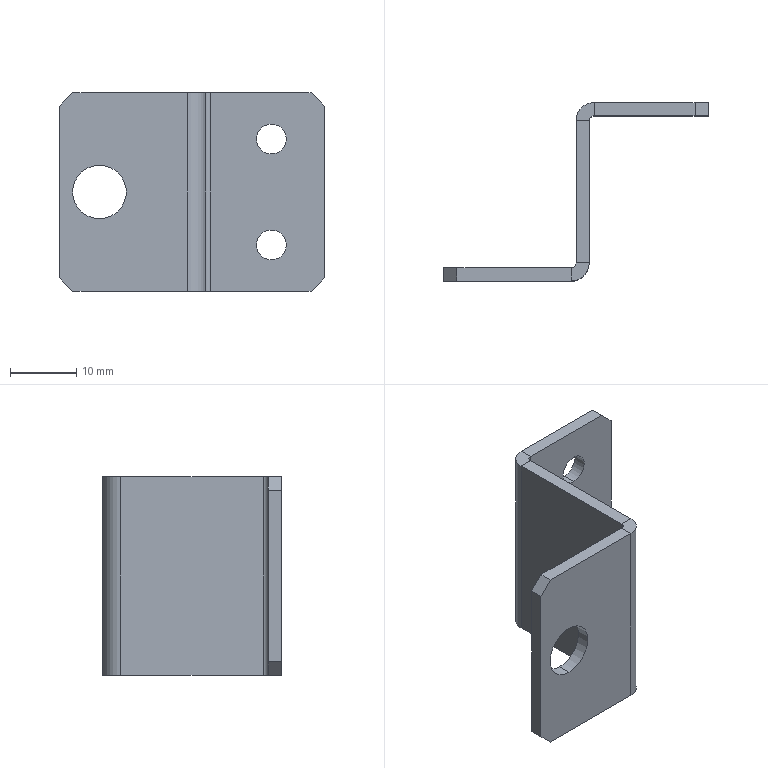Part | STEP file | 11-FG-SJ01211 | 1 solid | 32 faces | box 40 x 27 x 30 mm | volume 3628 mm3 | plane 22 | cylinder 10 | commonest cylinder face diameters 4.5 x4 1.473 x2 5.473 x2 8.1 x2
STEP:
#1=CARTESIAN_POINT('',(32.,23.,4.75));
#2=VERTEX_POINT('',#1);
#3=CARTESIAN_POINT('',(32.,23.,9.25));
#4=VERTEX_POINT('',#3);
#5=CARTESIAN_POINT('',(32.,23.,7.));
#6=DIRECTION('',(0.,1.,0.));
#7=DIRECTION('',(0.,0.,1.));
#8=AXIS2_PLACEMENT_3D('',#5,#6,#7);
#9=CIRCLE('',#8,2.25);
#10=EDGE_CURVE('',#2,#4,#9,.T.);
#11=ORIENTED_EDGE('',*,*,#10,.F.);
#12=CARTESIAN_POINT('',(32.,25.,4.75));
#13=VERTEX_POINT('',#12);
#14=CARTESIAN_POINT('',(32.,25.,4.75));
#15=DIRECTION('',(0.,1.,0.));
#16=VECTOR('',#15,1000.);
#17=LINE('',#14,#16);
#18=EDGE_CURVE('',#2,#13,#17,.T.);
#19=ORIENTED_EDGE('',*,*,#18,.T.);
#20=CARTESIAN_POINT('',(32.,25.,9.25));
#21=VERTEX_POINT('',#20);
#22=CARTESIAN_POINT('',(32.,25.,7.));
#23=DIRECTION('',(0.,1.,0.));
#24=DIRECTION('',(0.,0.,1.));
#25=AXIS2_PLACEMENT_3D('',#22,#23,#24);
#26=CIRCLE('',#25,2.25);
#27=EDGE_CURVE('',#13,#21,#26,.T.);
#28=ORIENTED_EDGE('',*,*,#27,.T.);
#29=CARTESIAN_POINT('',(32.,25.,9.25));
#30=DIRECTION('',(0.,1.,0.));
#31=VECTOR('',#30,1000.);
#32=LINE('',#29,#31);
#33=EDGE_CURVE('',#4,#21,#32,.T.);
#34=ORIENTED_EDGE('',*,*,#33,.F.);
#35=EDGE_LOOP('',(#11,#19,#28,#34));
#36=FACE_OUTER_BOUND('',#35,.T.);
#37=CARTESIAN_POINT('',(32.,25.,7.));
#38=DIRECTION('',(0.,1.,0.));
#39=DIRECTION('',(0.,0.,1.));
#40=AXIS2_PLACEMENT_3D('',#37,#38,#39);
#41=CYLINDRICAL_SURFACE('',#40,2.25);
#42=ADVANCED_FACE('',(#36),#41,.F.);
#43=CARTESIAN_POINT('',(32.,23.,20.75));
#44=VERTEX_POINT('',#43);
#45=CARTESIAN_POINT('',(32.,23.,25.25));
#46=VERTEX_POINT('',#45);
#47=CARTESIAN_POINT('',(32.,23.,23.));
#48=DIRECTION('',(0.,1.,0.));
#49=DIRECTION('',(0.,0.,1.));
#50=AXIS2_PLACEMENT_3D('',#47,#48,#49);
#51=CIRCLE('',#50,2.25);
#52=EDGE_CURVE('',#44,#46,#51,.T.);
#53=ORIENTED_EDGE('',*,*,#52,.F.);
#54=CARTESIAN_POINT('',(32.,25.,20.75));
#55=VERTEX_POINT('',#54);
#56=CARTESIAN_POINT('',(32.,25.,20.75));
#57=DIRECTION('',(0.,1.,0.));
#58=VECTOR('',#57,1000.);
#59=LINE('',#56,#58);
#60=EDGE_CURVE('',#44,#55,#59,.T.);
#61=ORIENTED_EDGE('',*,*,#60,.T.);
#62=CARTESIAN_POINT('',(32.,25.,25.25));
#63=VERTEX_POINT('',#62);
#64=CARTESIAN_POINT('',(32.,25.,23.));
#65=DIRECTION('',(0.,1.,0.));
#66=DIRECTION('',(0.,0.,1.));
#67=AXIS2_PLACEMENT_3D('',#64,#65,#66);
#68=CIRCLE('',#67,2.25);
#69=EDGE_CURVE('',#55,#63,#68,.T.);
#70=ORIENTED_EDGE('',*,*,#69,.T.);
#71=CARTESIAN_POINT('',(32.,25.,25.25));
#72=DIRECTION('',(0.,1.,0.));
#73=VECTOR('',#72,1000.);
#74=LINE('',#71,#73);
#75=EDGE_CURVE('',#46,#63,#74,.T.);
#76=ORIENTED_EDGE('',*,*,#75,.F.);
#77=EDGE_LOOP('',(#53,#61,#70,#76));
#78=FACE_OUTER_BOUND('',#77,.T.);
#79=CARTESIAN_POINT('',(32.,25.,23.));
#80=DIRECTION('',(0.,1.,0.));
#81=DIRECTION('',(0.,0.,1.));
#82=AXIS2_PLACEMENT_3D('',#79,#80,#81);
#83=CYLINDRICAL_SURFACE('',#82,2.25);
#84=ADVANCED_FACE('',(#78),#83,.F.);
#85=CARTESIAN_POINT('',(6.,0.,10.95));
#86=VERTEX_POINT('',#85);
#87=CARTESIAN_POINT('',(6.,0.,19.05));
#88=VERTEX_POINT('',#87);
#89=CARTESIAN_POINT('',(6.,0.,15.));
#90=DIRECTION('',(0.,1.,0.));
#91=DIRECTION('',(0.,0.,1.));
#92=AXIS2_PLACEMENT_3D('',#89,#90,#91);
#93=CIRCLE('',#92,4.05);
#94=EDGE_CURVE('',#86,#88,#93,.T.);
#95=ORIENTED_EDGE('',*,*,#94,.T.);
#96=CARTESIAN_POINT('',(6.,-2.,19.05));
#97=VERTEX_POINT('',#96);
#98=CARTESIAN_POINT('',(6.,8.,19.05));
#99=DIRECTION('',(0.,-1.,0.));
#100=VECTOR('',#99,1000.);
#101=LINE('',#98,#100);
#102=EDGE_CURVE('',#88,#97,#101,.T.);
#103=ORIENTED_EDGE('',*,*,#102,.T.);
#104=CARTESIAN_POINT('',(6.,-2.,10.95));
#105=VERTEX_POINT('',#104);
#106=CARTESIAN_POINT('',(6.,-2.,15.));
#107=DIRECTION('',(0.,-1.,0.));
#108=DIRECTION('',(0.,0.,-1.));
#109=AXIS2_PLACEMENT_3D('',#106,#107,#108);
#110=CIRCLE('',#109,4.05);
#111=EDGE_CURVE('',#97,#105,#110,.T.);
#112=ORIENTED_EDGE('',*,*,#111,.T.);
#113=CARTESIAN_POINT('',(6.,8.,10.95));
#114=DIRECTION('',(0.,-1.,0.));
#115=VECTOR('',#114,1000.);
#116=LINE('',#113,#115);
#117=EDGE_CURVE('',#86,#105,#116,.T.);
#118=ORIENTED_EDGE('',*,*,#117,.F.);
#119=EDGE_LOOP('',(#95,#103,#112,#118));
#120=FACE_OUTER_BOUND('',#119,.T.);
#121=CARTESIAN_POINT('',(6.,8.,15.));
#122=DIRECTION('',(0.,-1.,0.));
#123=DIRECTION('',(0.,0.,-1.));
#124=AXIS2_PLACEMENT_3D('',#121,#122,#123);
#125=CYLINDRICAL_SURFACE('',#124,4.05);
#126=ADVANCED_FACE('',(#120),#125,.F.);
#127=CARTESIAN_POINT('',(20.,0.7366,30.));
#128=VERTEX_POINT('',#127);
#129=CARTESIAN_POINT('',(22.,0.7366,30.));
#130=VERTEX_POINT('',#129);
#131=CARTESIAN_POINT('',(20.,0.7366,30.));
#132=DIRECTION('',(1.,0.,0.));
#133=VECTOR('',#132,1000.);
#134=LINE('',#131,#133);
#135=EDGE_CURVE('',#128,#130,#134,.T.);
#136=ORIENTED_EDGE('',*,*,#135,.F.);
#137=CARTESIAN_POINT('',(19.263,0.,30.));
#138=VERTEX_POINT('',#137);
#139=CARTESIAN_POINT('',(19.263,0.7366,30.));
#140=DIRECTION('',(0.,0.,1.));
#141=DIRECTION('',(-1.,0.,0.));
#142=AXIS2_PLACEMENT_3D('',#139,#140,#141);
#143=CIRCLE('',#142,0.7366);
#144=EDGE_CURVE('',#138,#128,#143,.T.);
#145=ORIENTED_EDGE('',*,*,#144,.F.);
#146=CARTESIAN_POINT('',(19.263,-2.,30.));
#147=VERTEX_POINT('',#146);
#148=CARTESIAN_POINT('',(19.263,-2.,30.));
#149=DIRECTION('',(0.,1.,0.));
#150=VECTOR('',#149,1000.);
#151=LINE('',#148,#150);
#152=EDGE_CURVE('',#147,#138,#151,.T.);
#153=ORIENTED_EDGE('',*,*,#152,.F.);
#154=CARTESIAN_POINT('',(19.263,0.7366,30.));
#155=DIRECTION('',(0.,0.,1.));
#156=DIRECTION('',(1.,0.,0.));
#157=AXIS2_PLACEMENT_3D('',#154,#155,#156);
#158=CIRCLE('',#157,2.737);
#159=EDGE_CURVE('',#147,#130,#158,.T.);
#160=ORIENTED_EDGE('',*,*,#159,.T.);
#161=EDGE_LOOP('',(#136,#145,#153,#160));
#162=FACE_OUTER_BOUND('',#161,.T.);
#163=CARTESIAN_POINT('',(20.,0.7366,30.));
#164=DIRECTION('',(0.,0.,1.));
#165=DIRECTION('',(1.,0.,0.));
#166=AXIS2_PLACEMENT_3D('',#163,#164,#165);
#167=PLANE('',#166);
#168=ADVANCED_FACE('',(#162),#167,.T.);
#169=CARTESIAN_POINT('',(20.,22.263,30.));
#170=VERTEX_POINT('',#169);
#171=CARTESIAN_POINT('',(20.,0.,30.));
#172=DIRECTION('',(0.,1.,0.));
#173=VECTOR('',#172,1000.);
#174=LINE('',#171,#173);
#175=EDGE_CURVE('',#128,#170,#174,.T.);
#176=ORIENTED_EDGE('',*,*,#175,.F.);
#177=ORIENTED_EDGE('',*,*,#135,.T.);
#178=CARTESIAN_POINT('',(22.,22.263,30.));
#179=VERTEX_POINT('',#178);
#180=CARTESIAN_POINT('',(22.,0.,30.));
#181=DIRECTION('',(0.,1.,0.));
#182=VECTOR('',#181,1000.);
#183=LINE('',#180,#182);
#184=EDGE_CURVE('',#130,#179,#183,.T.);
#185=ORIENTED_EDGE('',*,*,#184,.T.);
#186=CARTESIAN_POINT('',(22.,22.263,30.));
#187=DIRECTION('',(-1.,0.,0.));
#188=VECTOR('',#187,1000.);
#189=LINE('',#186,#188);
#190=EDGE_CURVE('',#179,#170,#189,.T.);
#191=ORIENTED_EDGE('',*,*,#190,.T.);
#192=EDGE_LOOP('',(#176,#177,#185,#191));
#193=FACE_OUTER_BOUND('',#192,.T.);
#194=CARTESIAN_POINT('',(19.263,-2.,30.));
#195=DIRECTION('',(0.,0.,1.));
#196=DIRECTION('',(1.,0.,0.));
#197=AXIS2_PLACEMENT_3D('',#194,#195,#196);
#198=PLANE('',#197);
#199=ADVANCED_FACE('',(#193),#198,.T.);
#200=CARTESIAN_POINT('',(19.263,0.,0.));
#201=VERTEX_POINT('',#200);
#202=CARTESIAN_POINT('',(19.263,-2.,0.));
#203=VERTEX_POINT('',#202);
#204=CARTESIAN_POINT('',(19.263,0.,0.));
#205=DIRECTION('',(0.,-1.,0.));
#206=VECTOR('',#205,1000.);
#207=LINE('',#204,#206);
#208=EDGE_CURVE('',#201,#203,#207,.T.);
#209=ORIENTED_EDGE('',*,*,#208,.F.);
#210=CARTESIAN_POINT('',(20.,0.7366,0.));
#211=VERTEX_POINT('',#210);
#212=CARTESIAN_POINT('',(19.263,0.7366,0.));
#213=DIRECTION('',(0.,0.,1.));
#214=DIRECTION('',(-1.,0.,0.));
#215=AXIS2_PLACEMENT_3D('',#212,#213,#214);
#216=CIRCLE('',#215,0.7366);
#217=EDGE_CURVE('',#201,#211,#216,.T.);
#218=ORIENTED_EDGE('',*,*,#217,.T.);
#219=CARTESIAN_POINT('',(22.,0.7366,0.));
#220=VERTEX_POINT('',#219);
#221=CARTESIAN_POINT('',(22.,0.7366,0.));
#222=DIRECTION('',(-1.,0.,0.));
#223=VECTOR('',#222,1000.);
#224=LINE('',#221,#223);
#225=EDGE_CURVE('',#220,#211,#224,.T.);
#226=ORIENTED_EDGE('',*,*,#225,.F.);
#227=CARTESIAN_POINT('',(19.263,0.7366,0.));
#228=DIRECTION('',(0.,0.,1.));
#229=DIRECTION('',(1.,0.,0.));
#230=AXIS2_PLACEMENT_3D('',#227,#228,#229);
#231=CIRCLE('',#230,2.737);
#232=EDGE_CURVE('',#203,#220,#231,.T.);
#233=ORIENTED_EDGE('',*,*,#232,.F.);
#234=EDGE_LOOP('',(#209,#218,#226,#233));
#235=FACE_OUTER_BOUND('',#234,.T.);
#236=CARTESIAN_POINT('',(19.263,0.,0.));
#237=DIRECTION('',(0.,0.,-1.));
#238=DIRECTION('',(-1.,0.,0.));
#239=AXIS2_PLACEMENT_3D('',#236,#237,#238);
#240=PLANE('',#239);
#241=ADVANCED_FACE('',(#235),#240,.T.);
#242=CARTESIAN_POINT('',(2.,-2.,0.));
#243=VERTEX_POINT('',#242);
#244=CARTESIAN_POINT('',(0.,-2.,0.));
#245=DIRECTION('',(1.,0.,0.));
#246=VECTOR('',#245,1000.);
#247=LINE('',#244,#246);
#248=EDGE_CURVE('',#243,#203,#247,.T.);
#249=ORIENTED_EDGE('',*,*,#248,.F.);
#250=CARTESIAN_POINT('',(2.,0.,0.));
#251=VERTEX_POINT('',#250);
#252=CARTESIAN_POINT('',(2.,0.7366,0.));
#253=DIRECTION('',(0.,1.,0.));
#254=VECTOR('',#253,1000.);
#255=LINE('',#252,#254);
#256=EDGE_CURVE('',#243,#251,#255,.T.);
#257=ORIENTED_EDGE('',*,*,#256,.T.);
#258=CARTESIAN_POINT('',(0.,0.,0.));
#259=DIRECTION('',(1.,0.,0.));
#260=VECTOR('',#259,1000.);
#261=LINE('',#258,#260);
#262=EDGE_CURVE('',#251,#201,#261,.T.);
#263=ORIENTED_EDGE('',*,*,#262,.T.);
#264=ORIENTED_EDGE('',*,*,#208,.T.);
#265=EDGE_LOOP('',(#249,#257,#263,#264));
#266=FACE_OUTER_BOUND('',#265,.T.);
#267=CARTESIAN_POINT('',(22.,0.7366,0.));
#268=DIRECTION('',(0.,0.,-1.));
#269=DIRECTION('',(-1.,0.,0.));
#270=AXIS2_PLACEMENT_3D('',#267,#268,#269);
#271=PLANE('',#270);
#272=ADVANCED_FACE('',(#266),#271,.T.);
#273=CARTESIAN_POINT('',(22.737,25.,30.));
#274=VERTEX_POINT('',#273);
#275=CARTESIAN_POINT('',(22.737,23.,30.));
#276=VERTEX_POINT('',#275);
#277=CARTESIAN_POINT('',(22.737,25.,30.));
#278=DIRECTION('',(0.,-1.,0.));
#279=VECTOR('',#278,1000.);
#280=LINE('',#277,#279);
#281=EDGE_CURVE('',#274,#276,#280,.T.);
#282=ORIENTED_EDGE('',*,*,#281,.F.);
#283=CARTESIAN_POINT('',(22.737,22.263,30.));
#284=DIRECTION('',(0.,0.,-1.));
#285=DIRECTION('',(1.,0.,0.));
#286=AXIS2_PLACEMENT_3D('',#283,#284,#285);
#287=CIRCLE('',#286,2.737);
#288=EDGE_CURVE('',#170,#274,#287,.T.);
#289=ORIENTED_EDGE('',*,*,#288,.F.);
#290=ORIENTED_EDGE('',*,*,#190,.F.);
#291=CARTESIAN_POINT('',(22.737,22.263,30.));
#292=DIRECTION('',(0.,0.,-1.));
#293=DIRECTION('',(1.,0.,0.));
#294=AXIS2_PLACEMENT_3D('',#291,#292,#293);
#295=CIRCLE('',#294,0.7366);
#296=EDGE_CURVE('',#179,#276,#295,.T.);
#297=ORIENTED_EDGE('',*,*,#296,.T.);
#298=EDGE_LOOP('',(#282,#289,#290,#297));
#299=FACE_OUTER_BOUND('',#298,.T.);
#300=CARTESIAN_POINT('',(22.737,25.,30.));
#301=DIRECTION('',(0.,0.,1.));
#302=DIRECTION('',(1.,0.,0.));
#303=AXIS2_PLACEMENT_3D('',#300,#301,#302);
#304=PLANE('',#303);
#305=ADVANCED_FACE('',(#299),#304,.T.);
#306=CARTESIAN_POINT('',(38.,23.,30.));
#307=VERTEX_POINT('',#306);
#308=CARTESIAN_POINT('',(20.,23.,30.));
#309=DIRECTION('',(1.,0.,0.));
#310=VECTOR('',#309,1000.);
#311=LINE('',#308,#310);
#312=EDGE_CURVE('',#276,#307,#311,.T.);
#313=ORIENTED_EDGE('',*,*,#312,.T.);
#314=CARTESIAN_POINT('',(38.,25.,30.));
#315=VERTEX_POINT('',#314);
#316=CARTESIAN_POINT('',(38.,22.263,30.));
#317=DIRECTION('',(0.,1.,0.));
#318=VECTOR('',#317,1000.);
#319=LINE('',#316,#318);
#320=EDGE_CURVE('',#307,#315,#319,.T.);
#321=ORIENTED_EDGE('',*,*,#320,.T.);
#322=CARTESIAN_POINT('',(20.,25.,30.));
#323=DIRECTION('',(1.,0.,0.));
#324=VECTOR('',#323,1000.);
#325=LINE('',#322,#324);
#326=EDGE_CURVE('',#274,#315,#325,.T.);
#327=ORIENTED_EDGE('',*,*,#326,.F.);
#328=ORIENTED_EDGE('',*,*,#281,.T.);
#329=EDGE_LOOP('',(#313,#321,#327,#328));
#330=FACE_OUTER_BOUND('',#329,.T.);
#331=CARTESIAN_POINT('',(22.,22.263,30.));
#332=DIRECTION('',(0.,0.,1.));
#333=DIRECTION('',(1.,0.,0.));
#334=AXIS2_PLACEMENT_3D('',#331,#332,#333);
#335=PLANE('',#334);
#336=ADVANCED_FACE('',(#330),#335,.T.);
#337=CARTESIAN_POINT('',(20.,22.263,0.));
#338=VERTEX_POINT('',#337);
#339=CARTESIAN_POINT('',(22.,22.263,0.));
#340=VERTEX_POINT('',#339);
#341=CARTESIAN_POINT('',(20.,22.263,0.));
#342=DIRECTION('',(1.,0.,0.));
#343=VECTOR('',#342,1000.);
#344=LINE('',#341,#343);
#345=EDGE_CURVE('',#338,#340,#344,.T.);
#346=ORIENTED_EDGE('',*,*,#345,.F.);
#347=CARTESIAN_POINT('',(22.737,25.,0.));
#348=VERTEX_POINT('',#347);
#349=CARTESIAN_POINT('',(22.737,22.263,0.));
#350=DIRECTION('',(0.,0.,-1.));
#351=DIRECTION('',(1.,0.,0.));
#352=AXIS2_PLACEMENT_3D('',#349,#350,#351);
#353=CIRCLE('',#352,2.737);
#354=EDGE_CURVE('',#338,#348,#353,.T.);
#355=ORIENTED_EDGE('',*,*,#354,.T.);
#356=CARTESIAN_POINT('',(22.737,23.,0.));
#357=VERTEX_POINT('',#356);
#358=CARTESIAN_POINT('',(22.737,23.,0.));
#359=DIRECTION('',(0.,1.,0.));
#360=VECTOR('',#359,1000.);
#361=LINE('',#358,#360);
#362=EDGE_CURVE('',#357,#348,#361,.T.);
#363=ORIENTED_EDGE('',*,*,#362,.F.);
#364=CARTESIAN_POINT('',(22.737,22.263,0.));
#365=DIRECTION('',(0.,0.,-1.));
#366=DIRECTION('',(1.,0.,0.));
#367=AXIS2_PLACEMENT_3D('',#364,#365,#366);
#368=CIRCLE('',#367,0.7366);
#369=EDGE_CURVE('',#340,#357,#368,.T.);
#370=ORIENTED_EDGE('',*,*,#369,.F.);
#371=EDGE_LOOP('',(#346,#355,#363,#370));
#372=FACE_OUTER_BOUND('',#371,.T.);
#373=CARTESIAN_POINT('',(20.,22.263,0.));
#374=DIRECTION('',(0.,0.,-1.));
#375=DIRECTION('',(-1.,0.,0.));
#376=AXIS2_PLACEMENT_3D('',#373,#374,#375);
#377=PLANE('',#376);
#378=ADVANCED_FACE('',(#372),#377,.T.);
#379=CARTESIAN_POINT('',(20.,0.,0.));
#380=DIRECTION('',(0.,1.,0.));
#381=VECTOR('',#380,1000.);
#382=LINE('',#379,#381);
#383=EDGE_CURVE('',#211,#338,#382,.T.);
#384=ORIENTED_EDGE('',*,*,#383,.T.);
#385=ORIENTED_EDGE('',*,*,#345,.T.);
#386=CARTESIAN_POINT('',(22.,0.,0.));
#387=DIRECTION('',(0.,1.,0.));
#388=VECTOR('',#387,1000.);
#389=LINE('',#386,#388);
#390=EDGE_CURVE('',#220,#340,#389,.T.);
#391=ORIENTED_EDGE('',*,*,#390,.F.);
#392=ORIENTED_EDGE('',*,*,#225,.T.);
#393=EDGE_LOOP('',(#384,#385,#391,#392));
#394=FACE_OUTER_BOUND('',#393,.T.);
#395=CARTESIAN_POINT('',(22.737,23.,0.));
#396=DIRECTION('',(0.,0.,-1.));
#397=DIRECTION('',(-1.,0.,0.));
#398=AXIS2_PLACEMENT_3D('',#395,#396,#397);
#399=PLANE('',#398);
#400=ADVANCED_FACE('',(#394),#399,.T.);
#401=CARTESIAN_POINT('',(32.,23.,7.));
#402=DIRECTION('',(0.,1.,0.));
#403=DIRECTION('',(0.,0.,1.));
#404=AXIS2_PLACEMENT_3D('',#401,#402,#403);
#405=CIRCLE('',#404,2.25);
#406=EDGE_CURVE('',#4,#2,#405,.T.);
#407=ORIENTED_EDGE('',*,*,#406,.T.);
#408=ORIENTED_EDGE('',*,*,#10,.T.);
#409=EDGE_LOOP('',(#407,#408));
#410=FACE_BOUND('',#409,.T.);
#411=CARTESIAN_POINT('',(32.,23.,23.));
#412=DIRECTION('',(0.,1.,0.));
#413=DIRECTION('',(0.,0.,1.));
#414=AXIS2_PLACEMENT_3D('',#411,#412,#413);
#415=CIRCLE('',#414,2.25);
#416=EDGE_CURVE('',#46,#44,#415,.T.);
#417=ORIENTED_EDGE('',*,*,#416,.T.);
#418=ORIENTED_EDGE('',*,*,#52,.T.);
#419=EDGE_LOOP('',(#417,#418));
#420=FACE_BOUND('',#419,.T.);
#421=CARTESIAN_POINT('',(38.,23.,0.));
#422=VERTEX_POINT('',#421);
#423=CARTESIAN_POINT('',(20.,23.,0.));
#424=DIRECTION('',(1.,0.,0.));
#425=VECTOR('',#424,1000.);
#426=LINE('',#423,#425);
#427=EDGE_CURVE('',#357,#422,#426,.T.);
#428=ORIENTED_EDGE('',*,*,#427,.T.);
#429=CARTESIAN_POINT('',(40.,23.,2.));
#430=VERTEX_POINT('',#429);
#431=CARTESIAN_POINT('',(38.,23.,0.));
#432=DIRECTION('',(0.7071,0.,0.7071));
#433=VECTOR('',#432,1000.);
#434=LINE('',#431,#433);
#435=EDGE_CURVE('',#422,#430,#434,.T.);
#436=ORIENTED_EDGE('',*,*,#435,.T.);
#437=CARTESIAN_POINT('',(40.,23.,28.));
#438=VERTEX_POINT('',#437);
#439=CARTESIAN_POINT('',(40.,23.,30.));
#440=DIRECTION('',(0.,0.,-1.));
#441=VECTOR('',#440,1000.);
#442=LINE('',#439,#441);
#443=EDGE_CURVE('',#438,#430,#442,.T.);
#444=ORIENTED_EDGE('',*,*,#443,.F.);
#445=CARTESIAN_POINT('',(40.,23.,28.));
#446=DIRECTION('',(-0.7071,0.,0.7071));
#447=VECTOR('',#446,1000.);
#448=LINE('',#445,#447);
#449=EDGE_CURVE('',#438,#307,#448,.T.);
#450=ORIENTED_EDGE('',*,*,#449,.T.);
#451=ORIENTED_EDGE('',*,*,#312,.F.);
#452=CARTESIAN_POINT('',(22.737,23.,30.));
#453=DIRECTION('',(0.,0.,-1.));
#454=VECTOR('',#453,1000.);
#455=LINE('',#452,#454);
#456=EDGE_CURVE('',#276,#357,#455,.T.);
#457=ORIENTED_EDGE('',*,*,#456,.T.);
#458=EDGE_LOOP('',(#428,#436,#444,#450,#451,#457));
#459=FACE_OUTER_BOUND('',#458,.T.);
#460=CARTESIAN_POINT('',(20.,23.,30.));
#461=DIRECTION('',(0.,1.,0.));
#462=DIRECTION('',(0.,0.,1.));
#463=AXIS2_PLACEMENT_3D('',#460,#461,#462);
#464=PLANE('',#463);
#465=ADVANCED_FACE('',(#410,#420,#459),#464,.F.);
#466=ORIENTED_EDGE('',*,*,#443,.T.);
#467=CARTESIAN_POINT('',(40.,25.,2.));
#468=VERTEX_POINT('',#467);
#469=CARTESIAN_POINT('',(40.,25.,2.));
#470=DIRECTION('',(0.,1.,0.));
#471=VECTOR('',#470,1000.);
#472=LINE('',#469,#471);
#473=EDGE_CURVE('',#430,#468,#472,.T.);
#474=ORIENTED_EDGE('',*,*,#473,.T.);
#475=CARTESIAN_POINT('',(40.,25.,28.));
#476=VERTEX_POINT('',#475);
#477=CARTESIAN_POINT('',(40.,25.,30.));
#478=DIRECTION('',(0.,0.,-1.));
#479=VECTOR('',#478,1000.);
#480=LINE('',#477,#479);
#481=EDGE_CURVE('',#476,#468,#480,.T.);
#482=ORIENTED_EDGE('',*,*,#481,.F.);
#483=CARTESIAN_POINT('',(40.,25.,28.));
#484=DIRECTION('',(0.,-1.,0.));
#485=VECTOR('',#484,1000.);
#486=LINE('',#483,#485);
#487=EDGE_CURVE('',#476,#438,#486,.T.);
#488=ORIENTED_EDGE('',*,*,#487,.T.);
#489=EDGE_LOOP('',(#466,#474,#482,#488));
#490=FACE_OUTER_BOUND('',#489,.T.);
#491=CARTESIAN_POINT('',(40.,25.,30.));
#492=DIRECTION('',(1.,0.,0.));
#493=DIRECTION('',(0.,0.,-1.));
#494=AXIS2_PLACEMENT_3D('',#491,#492,#493);
#495=PLANE('',#494);
#496=ADVANCED_FACE('',(#490),#495,.T.);
#497=CARTESIAN_POINT('',(32.,25.,7.));
#498=DIRECTION('',(0.,1.,0.));
#499=DIRECTION('',(0.,0.,1.));
#500=AXIS2_PLACEMENT_3D('',#497,#498,#499);
#501=CIRCLE('',#500,2.25);
#502=EDGE_CURVE('',#21,#13,#501,.T.);
#503=ORIENTED_EDGE('',*,*,#502,.F.);
#504=ORIENTED_EDGE('',*,*,#27,.F.);
#505=EDGE_LOOP('',(#503,#504));
#506=FACE_BOUND('',#505,.T.);
#507=CARTESIAN_POINT('',(32.,25.,23.));
#508=DIRECTION('',(0.,1.,0.));
#509=DIRECTION('',(0.,0.,1.));
#510=AXIS2_PLACEMENT_3D('',#507,#508,#509);
#511=CIRCLE('',#510,2.25);
#512=EDGE_CURVE('',#63,#55,#511,.T.);
#513=ORIENTED_EDGE('',*,*,#512,.F.);
#514=ORIENTED_EDGE('',*,*,#69,.F.);
#515=EDGE_LOOP('',(#513,#514));
#516=FACE_BOUND('',#515,.T.);
#517=ORIENTED_EDGE('',*,*,#481,.T.);
#518=CARTESIAN_POINT('',(38.,25.,0.));
#519=VERTEX_POINT('',#518);
#520=CARTESIAN_POINT('',(44.,25.,6.));
#521=DIRECTION('',(-0.7071,0.,-0.7071));
#522=VECTOR('',#521,1000.);
#523=LINE('',#520,#522);
#524=EDGE_CURVE('',#468,#519,#523,.T.);
#525=ORIENTED_EDGE('',*,*,#524,.T.);
#526=CARTESIAN_POINT('',(20.,25.,0.));
#527=DIRECTION('',(1.,0.,0.));
#528=VECTOR('',#527,1000.);
#529=LINE('',#526,#528);
#530=EDGE_CURVE('',#348,#519,#529,.T.);
#531=ORIENTED_EDGE('',*,*,#530,.F.);
#532=CARTESIAN_POINT('',(22.737,25.,30.));
#533=DIRECTION('',(0.,0.,-1.));
#534=VECTOR('',#533,1000.);
#535=LINE('',#532,#534);
#536=EDGE_CURVE('',#274,#348,#535,.T.);
#537=ORIENTED_EDGE('',*,*,#536,.F.);
#538=ORIENTED_EDGE('',*,*,#326,.T.);
#539=CARTESIAN_POINT('',(29.,25.,39.));
#540=DIRECTION('',(0.7071,0.,-0.7071));
#541=VECTOR('',#540,1000.);
#542=LINE('',#539,#541);
#543=EDGE_CURVE('',#315,#476,#542,.T.);
#544=ORIENTED_EDGE('',*,*,#543,.T.);
#545=EDGE_LOOP('',(#517,#525,#531,#537,#538,#544));
#546=FACE_OUTER_BOUND('',#545,.T.);
#547=CARTESIAN_POINT('',(20.,25.,30.));
#548=DIRECTION('',(0.,1.,0.));
#549=DIRECTION('',(0.,0.,1.));
#550=AXIS2_PLACEMENT_3D('',#547,#548,#549);
#551=PLANE('',#550);
#552=ADVANCED_FACE('',(#506,#516,#546),#551,.T.);
#553=ORIENTED_EDGE('',*,*,#354,.F.);
#554=CARTESIAN_POINT('',(20.,22.263,30.));
#555=DIRECTION('',(0.,0.,-1.));
#556=VECTOR('',#555,1000.);
#557=LINE('',#554,#556);
#558=EDGE_CURVE('',#170,#338,#557,.T.);
#559=ORIENTED_EDGE('',*,*,#558,.F.);
#560=ORIENTED_EDGE('',*,*,#288,.T.);
#561=ORIENTED_EDGE('',*,*,#536,.T.);
#562=EDGE_LOOP('',(#553,#559,#560,#561));
#563=FACE_OUTER_BOUND('',#562,.T.);
#564=CARTESIAN_POINT('',(22.737,22.263,30.));
#565=DIRECTION('',(0.,0.,-1.));
#566=DIRECTION('',(-1.,0.,0.));
#567=AXIS2_PLACEMENT_3D('',#564,#565,#566);
#568=CYLINDRICAL_SURFACE('',#567,2.737);
#569=ADVANCED_FACE('',(#563),#568,.T.);
#570=ORIENTED_EDGE('',*,*,#383,.F.);
#571=CARTESIAN_POINT('',(20.,0.7366,30.));
#572=DIRECTION('',(0.,0.,-1.));
#573=VECTOR('',#572,1000.);
#574=LINE('',#571,#573);
#575=EDGE_CURVE('',#128,#211,#574,.T.);
#576=ORIENTED_EDGE('',*,*,#575,.F.);
#577=ORIENTED_EDGE('',*,*,#175,.T.);
#578=ORIENTED_EDGE('',*,*,#558,.T.);
#579=EDGE_LOOP('',(#570,#576,#577,#578));
#580=FACE_OUTER_BOUND('',#579,.T.);
#581=CARTESIAN_POINT('',(20.,0.,30.));
#582=DIRECTION('',(-1.,0.,0.));
#583=DIRECTION('',(0.,0.,1.));
#584=AXIS2_PLACEMENT_3D('',#581,#582,#583);
#585=PLANE('',#584);
#586=ADVANCED_FACE('',(#580),#585,.T.);
#587=ORIENTED_EDGE('',*,*,#217,.F.);
#588=CARTESIAN_POINT('',(19.263,0.,30.));
#589=DIRECTION('',(0.,0.,-1.));
#590=VECTOR('',#589,1000.);
#591=LINE('',#588,#590);
#592=EDGE_CURVE('',#138,#201,#591,.T.);
#593=ORIENTED_EDGE('',*,*,#592,.F.);
#594=ORIENTED_EDGE('',*,*,#144,.T.);
#595=ORIENTED_EDGE('',*,*,#575,.T.);
#596=EDGE_LOOP('',(#587,#593,#594,#595));
#597=FACE_OUTER_BOUND('',#596,.T.);
#598=CARTESIAN_POINT('',(19.263,0.7366,30.));
#599=DIRECTION('',(0.,0.,-1.));
#600=DIRECTION('',(-1.,0.,0.));
#601=AXIS2_PLACEMENT_3D('',#598,#599,#600);
#602=CYLINDRICAL_SURFACE('',#601,0.7366);
#603=ADVANCED_FACE('',(#597),#602,.F.);
#604=ORIENTED_EDGE('',*,*,#94,.F.);
#605=CARTESIAN_POINT('',(6.,0.,15.));
#606=DIRECTION('',(0.,1.,0.));
#607=DIRECTION('',(0.,0.,1.));
#608=AXIS2_PLACEMENT_3D('',#605,#606,#607);
#609=CIRCLE('',#608,4.05);
#610=EDGE_CURVE('',#88,#86,#609,.T.);
#611=ORIENTED_EDGE('',*,*,#610,.F.);
#612=EDGE_LOOP('',(#604,#611));
#613=FACE_BOUND('',#612,.T.);
#614=ORIENTED_EDGE('',*,*,#262,.F.);
#615=CARTESIAN_POINT('',(0.,0.,2.));
#616=VERTEX_POINT('',#615);
#617=CARTESIAN_POINT('',(-14.,0.,16.));
#618=DIRECTION('',(-0.7071,0.,0.7071));
#619=VECTOR('',#618,1000.);
#620=LINE('',#617,#619);
#621=EDGE_CURVE('',#251,#616,#620,.T.);
#622=ORIENTED_EDGE('',*,*,#621,.T.);
#623=CARTESIAN_POINT('',(0.,0.,28.));
#624=VERTEX_POINT('',#623);
#625=CARTESIAN_POINT('',(0.,0.,30.));
#626=DIRECTION('',(0.,0.,-1.));
#627=VECTOR('',#626,1000.);
#628=LINE('',#625,#627);
#629=EDGE_CURVE('',#624,#616,#628,.T.);
#630=ORIENTED_EDGE('',*,*,#629,.F.);
#631=CARTESIAN_POINT('',(2.,0.,30.));
#632=VERTEX_POINT('',#631);
#633=CARTESIAN_POINT('',(1.,0.,29.));
#634=DIRECTION('',(0.7071,0.,0.7071));
#635=VECTOR('',#634,1000.);
#636=LINE('',#633,#635);
#637=EDGE_CURVE('',#624,#632,#636,.T.);
#638=ORIENTED_EDGE('',*,*,#637,.T.);
#639=CARTESIAN_POINT('',(0.,0.,30.));
#640=DIRECTION('',(1.,0.,0.));
#641=VECTOR('',#640,1000.);
#642=LINE('',#639,#641);
#643=EDGE_CURVE('',#632,#138,#642,.T.);
#644=ORIENTED_EDGE('',*,*,#643,.T.);
#645=ORIENTED_EDGE('',*,*,#592,.T.);
#646=EDGE_LOOP('',(#614,#622,#630,#638,#644,#645));
#647=FACE_OUTER_BOUND('',#646,.T.);
#648=CARTESIAN_POINT('',(0.,0.,30.));
#649=DIRECTION('',(0.,1.,0.));
#650=DIRECTION('',(0.,0.,1.));
#651=AXIS2_PLACEMENT_3D('',#648,#649,#650);
#652=PLANE('',#651);
#653=ADVANCED_FACE('',(#613,#647),#652,.T.);
#654=ORIENTED_EDGE('',*,*,#629,.T.);
#655=CARTESIAN_POINT('',(0.,-2.,2.));
#656=VERTEX_POINT('',#655);
#657=CARTESIAN_POINT('',(0.,-2.,2.));
#658=DIRECTION('',(0.,-1.,0.));
#659=VECTOR('',#658,1000.);
#660=LINE('',#657,#659);
#661=EDGE_CURVE('',#616,#656,#660,.T.);
#662=ORIENTED_EDGE('',*,*,#661,.T.);
#663=CARTESIAN_POINT('',(0.,-2.,28.));
#664=VERTEX_POINT('',#663);
#665=CARTESIAN_POINT('',(0.,-2.,30.));
#666=DIRECTION('',(0.,0.,-1.));
#667=VECTOR('',#666,1000.);
#668=LINE('',#665,#667);
#669=EDGE_CURVE('',#664,#656,#668,.T.);
#670=ORIENTED_EDGE('',*,*,#669,.F.);
#671=CARTESIAN_POINT('',(0.,-2.,28.));
#672=DIRECTION('',(0.,1.,0.));
#673=VECTOR('',#672,1000.);
#674=LINE('',#671,#673);
#675=EDGE_CURVE('',#664,#624,#674,.T.);
#676=ORIENTED_EDGE('',*,*,#675,.T.);
#677=EDGE_LOOP('',(#654,#662,#670,#676));
#678=FACE_OUTER_BOUND('',#677,.T.);
#679=CARTESIAN_POINT('',(0.,-2.,30.));
#680=DIRECTION('',(-1.,0.,0.));
#681=DIRECTION('',(0.,0.,1.));
#682=AXIS2_PLACEMENT_3D('',#679,#680,#681);
#683=PLANE('',#682);
#684=ADVANCED_FACE('',(#678),#683,.T.);
#685=CARTESIAN_POINT('',(6.,-2.,15.));
#686=DIRECTION('',(0.,-1.,0.));
#687=DIRECTION('',(0.,0.,-1.));
#688=AXIS2_PLACEMENT_3D('',#685,#686,#687);
#689=CIRCLE('',#688,4.05);
#690=EDGE_CURVE('',#105,#97,#689,.T.);
#691=ORIENTED_EDGE('',*,*,#690,.F.);
#692=ORIENTED_EDGE('',*,*,#111,.F.);
#693=EDGE_LOOP('',(#691,#692));
#694=FACE_BOUND('',#693,.T.);
#695=ORIENTED_EDGE('',*,*,#669,.T.);
#696=CARTESIAN_POINT('',(2.,-2.,0.));
#697=DIRECTION('',(0.7071,0.,-0.7071));
#698=VECTOR('',#697,1000.);
#699=LINE('',#696,#698);
#700=EDGE_CURVE('',#656,#243,#699,.T.);
#701=ORIENTED_EDGE('',*,*,#700,.T.);
#702=ORIENTED_EDGE('',*,*,#248,.T.);
#703=CARTESIAN_POINT('',(19.263,-2.,30.));
#704=DIRECTION('',(0.,0.,-1.));
#705=VECTOR('',#704,1000.);
#706=LINE('',#703,#705);
#707=EDGE_CURVE('',#147,#203,#706,.T.);
#708=ORIENTED_EDGE('',*,*,#707,.F.);
#709=CARTESIAN_POINT('',(2.,-2.,30.));
#710=VERTEX_POINT('',#709);
#711=CARTESIAN_POINT('',(0.,-2.,30.));
#712=DIRECTION('',(1.,0.,0.));
#713=VECTOR('',#712,1000.);
#714=LINE('',#711,#713);
#715=EDGE_CURVE('',#710,#147,#714,.T.);
#716=ORIENTED_EDGE('',*,*,#715,.F.);
#717=CARTESIAN_POINT('',(0.,-2.,28.));
#718=DIRECTION('',(-0.7071,0.,-0.7071));
#719=VECTOR('',#718,1000.);
#720=LINE('',#717,#719);
#721=EDGE_CURVE('',#710,#664,#720,.T.);
#722=ORIENTED_EDGE('',*,*,#721,.T.);
#723=EDGE_LOOP('',(#695,#701,#702,#708,#716,#722));
#724=FACE_OUTER_BOUND('',#723,.T.);
#725=CARTESIAN_POINT('',(0.,-2.,30.));
#726=DIRECTION('',(0.,1.,0.));
#727=DIRECTION('',(0.,0.,1.));
#728=AXIS2_PLACEMENT_3D('',#725,#726,#727);
#729=PLANE('',#728);
#730=ADVANCED_FACE('',(#694,#724),#729,.F.);
#731=ORIENTED_EDGE('',*,*,#232,.T.);
#732=CARTESIAN_POINT('',(22.,0.7366,30.));
#733=DIRECTION('',(0.,0.,-1.));
#734=VECTOR('',#733,1000.);
#735=LINE('',#732,#734);
#736=EDGE_CURVE('',#130,#220,#735,.T.);
#737=ORIENTED_EDGE('',*,*,#736,.F.);
#738=ORIENTED_EDGE('',*,*,#159,.F.);
#739=ORIENTED_EDGE('',*,*,#707,.T.);
#740=EDGE_LOOP('',(#731,#737,#738,#739));
#741=FACE_OUTER_BOUND('',#740,.T.);
#742=CARTESIAN_POINT('',(19.263,0.7366,30.));
#743=DIRECTION('',(0.,0.,-1.));
#744=DIRECTION('',(-1.,0.,0.));
#745=AXIS2_PLACEMENT_3D('',#742,#743,#744);
#746=CYLINDRICAL_SURFACE('',#745,2.737);
#747=ADVANCED_FACE('',(#741),#746,.T.);
#748=ORIENTED_EDGE('',*,*,#390,.T.);
#749=CARTESIAN_POINT('',(22.,22.263,30.));
#750=DIRECTION('',(0.,0.,-1.));
#751=VECTOR('',#750,1000.);
#752=LINE('',#749,#751);
#753=EDGE_CURVE('',#179,#340,#752,.T.);
#754=ORIENTED_EDGE('',*,*,#753,.F.);
#755=ORIENTED_EDGE('',*,*,#184,.F.);
#756=ORIENTED_EDGE('',*,*,#736,.T.);
#757=EDGE_LOOP('',(#748,#754,#755,#756));
#758=FACE_OUTER_BOUND('',#757,.T.);
#759=CARTESIAN_POINT('',(22.,0.,30.));
#760=DIRECTION('',(-1.,0.,0.));
#761=DIRECTION('',(0.,0.,1.));
#762=AXIS2_PLACEMENT_3D('',#759,#760,#761);
#763=PLANE('',#762);
#764=ADVANCED_FACE('',(#758),#763,.F.);
#765=ORIENTED_EDGE('',*,*,#369,.T.);
#766=ORIENTED_EDGE('',*,*,#456,.F.);
#767=ORIENTED_EDGE('',*,*,#296,.F.);
#768=ORIENTED_EDGE('',*,*,#753,.T.);
#769=EDGE_LOOP('',(#765,#766,#767,#768));
#770=FACE_OUTER_BOUND('',#769,.T.);
#771=CARTESIAN_POINT('',(22.737,22.263,30.));
#772=DIRECTION('',(0.,0.,-1.));
#773=DIRECTION('',(-1.,0.,0.));
#774=AXIS2_PLACEMENT_3D('',#771,#772,#773);
#775=CYLINDRICAL_SURFACE('',#774,0.7366);
#776=ADVANCED_FACE('',(#770),#775,.F.);
#777=ORIENTED_EDGE('',*,*,#643,.F.);
#778=CARTESIAN_POINT('',(2.,22.263,30.));
#779=DIRECTION('',(0.,-1.,0.));
#780=VECTOR('',#779,1000.);
#781=LINE('',#778,#780);
#782=EDGE_CURVE('',#632,#710,#781,.T.);
#783=ORIENTED_EDGE('',*,*,#782,.T.);
#784=ORIENTED_EDGE('',*,*,#715,.T.);
#785=ORIENTED_EDGE('',*,*,#152,.T.);
#786=EDGE_LOOP('',(#777,#783,#784,#785));
#787=FACE_OUTER_BOUND('',#786,.T.);
#788=CARTESIAN_POINT('',(22.737,22.263,30.));
#789=DIRECTION('',(0.,0.,1.));
#790=DIRECTION('',(1.,0.,0.));
#791=AXIS2_PLACEMENT_3D('',#788,#789,#790);
#792=PLANE('',#791);
#793=ADVANCED_FACE('',(#787),#792,.T.);
#794=ORIENTED_EDGE('',*,*,#530,.T.);
#795=CARTESIAN_POINT('',(38.,23.,0.));
#796=DIRECTION('',(0.,-1.,0.));
#797=VECTOR('',#796,1000.);
#798=LINE('',#795,#797);
#799=EDGE_CURVE('',#519,#422,#798,.T.);
#800=ORIENTED_EDGE('',*,*,#799,.T.);
#801=ORIENTED_EDGE('',*,*,#427,.F.);
#802=ORIENTED_EDGE('',*,*,#362,.T.);
#803=EDGE_LOOP('',(#794,#800,#801,#802));
#804=FACE_OUTER_BOUND('',#803,.T.);
#805=CARTESIAN_POINT('',(22.737,22.263,0.));
#806=DIRECTION('',(0.,0.,1.));
#807=DIRECTION('',(1.,0.,0.));
#808=AXIS2_PLACEMENT_3D('',#805,#806,#807);
#809=PLANE('',#808);
#810=ADVANCED_FACE('',(#804),#809,.F.);
#811=ORIENTED_EDGE('',*,*,#102,.F.);
#812=ORIENTED_EDGE('',*,*,#610,.T.);
#813=ORIENTED_EDGE('',*,*,#117,.T.);
#814=ORIENTED_EDGE('',*,*,#690,.T.);
#815=EDGE_LOOP('',(#811,#812,#813,#814));
#816=FACE_OUTER_BOUND('',#815,.T.);
#817=CARTESIAN_POINT('',(6.,8.,15.));
#818=DIRECTION('',(0.,-1.,0.));
#819=DIRECTION('',(0.,0.,-1.));
#820=AXIS2_PLACEMENT_3D('',#817,#818,#819);
#821=CYLINDRICAL_SURFACE('',#820,4.05);
#822=ADVANCED_FACE('',(#816),#821,.F.);
#823=ORIENTED_EDGE('',*,*,#700,.F.);
#824=ORIENTED_EDGE('',*,*,#661,.F.);
#825=ORIENTED_EDGE('',*,*,#621,.F.);
#826=ORIENTED_EDGE('',*,*,#256,.F.);
#827=EDGE_LOOP('',(#823,#824,#825,#826));
#828=FACE_OUTER_BOUND('',#827,.T.);
#829=CARTESIAN_POINT('',(2.,0.7366,0.));
#830=DIRECTION('',(0.7071,0.,0.7071));
#831=DIRECTION('',(0.,1.,0.));
#832=AXIS2_PLACEMENT_3D('',#829,#830,#831);
#833=PLANE('',#832);
#834=ADVANCED_FACE('',(#828),#833,.F.);
#835=ORIENTED_EDGE('',*,*,#721,.F.);
#836=ORIENTED_EDGE('',*,*,#782,.F.);
#837=ORIENTED_EDGE('',*,*,#637,.F.);
#838=ORIENTED_EDGE('',*,*,#675,.F.);
#839=EDGE_LOOP('',(#835,#836,#837,#838));
#840=FACE_OUTER_BOUND('',#839,.T.);
#841=CARTESIAN_POINT('',(0.,-2.,28.));
#842=DIRECTION('',(0.7071,0.,-0.7071));
#843=DIRECTION('',(0.,1.,0.));
#844=AXIS2_PLACEMENT_3D('',#841,#842,#843);
#845=PLANE('',#844);
#846=ADVANCED_FACE('',(#840),#845,.F.);
#847=ORIENTED_EDGE('',*,*,#524,.F.);
#848=ORIENTED_EDGE('',*,*,#473,.F.);
#849=ORIENTED_EDGE('',*,*,#435,.F.);
#850=ORIENTED_EDGE('',*,*,#799,.F.);
#851=EDGE_LOOP('',(#847,#848,#849,#850));
#852=FACE_OUTER_BOUND('',#851,.T.);
#853=CARTESIAN_POINT('',(38.,22.263,0.));
#854=DIRECTION('',(0.7071,0.,-0.7071));
#855=DIRECTION('',(0.,1.,0.));
#856=AXIS2_PLACEMENT_3D('',#853,#854,#855);
#857=PLANE('',#856);
#858=ADVANCED_FACE('',(#852),#857,.T.);
#859=ORIENTED_EDGE('',*,*,#543,.F.);
#860=ORIENTED_EDGE('',*,*,#320,.F.);
#861=ORIENTED_EDGE('',*,*,#449,.F.);
#862=ORIENTED_EDGE('',*,*,#487,.F.);
#863=EDGE_LOOP('',(#859,#860,#861,#862));
#864=FACE_OUTER_BOUND('',#863,.T.);
#865=CARTESIAN_POINT('',(40.,25.,28.));
#866=DIRECTION('',(-0.7071,0.,-0.7071));
#867=DIRECTION('',(0.,-1.,0.));
#868=AXIS2_PLACEMENT_3D('',#865,#866,#867);
#869=PLANE('',#868);
#870=ADVANCED_FACE('',(#864),#869,.F.);
#871=ORIENTED_EDGE('',*,*,#60,.F.);
#872=ORIENTED_EDGE('',*,*,#416,.F.);
#873=ORIENTED_EDGE('',*,*,#75,.T.);
#874=ORIENTED_EDGE('',*,*,#512,.T.);
#875=EDGE_LOOP('',(#871,#872,#873,#874));
#876=FACE_OUTER_BOUND('',#875,.T.);
#877=CARTESIAN_POINT('',(32.,25.,23.));
#878=DIRECTION('',(0.,1.,0.));
#879=DIRECTION('',(0.,0.,1.));
#880=AXIS2_PLACEMENT_3D('',#877,#878,#879);
#881=CYLINDRICAL_SURFACE('',#880,2.25);
#882=ADVANCED_FACE('',(#876),#881,.F.);
#883=ORIENTED_EDGE('',*,*,#18,.F.);
#884=ORIENTED_EDGE('',*,*,#406,.F.);
#885=ORIENTED_EDGE('',*,*,#33,.T.);
#886=ORIENTED_EDGE('',*,*,#502,.T.);
#887=EDGE_LOOP('',(#883,#884,#885,#886));
#888=FACE_OUTER_BOUND('',#887,.T.);
#889=CARTESIAN_POINT('',(32.,25.,7.));
#890=DIRECTION('',(0.,1.,0.));
#891=DIRECTION('',(0.,0.,1.));
#892=AXIS2_PLACEMENT_3D('',#889,#890,#891);
#893=CYLINDRICAL_SURFACE('',#892,2.25);
#894=ADVANCED_FACE('',(#888),#893,.F.);
#895=CLOSED_SHELL('',(#42,#84,#126,#168,#199,#241,#272,#305,#336,#378,#400,#465,#496,#552,#569,#586,#603,#653,#684,#730,#747,#764,#776,#793,#810,#822,#834,#846,#858,#870,#882,#894));
#896=MANIFOLD_SOLID_BREP('',#895);
#897=CARTESIAN_POINT('',(0.,0.,0.));
#898=DIRECTION('',(0.,0.,1.));
#899=DIRECTION('',(1.,0.,0.));
#900=AXIS2_PLACEMENT_3D('',#897,#898,#899);
#901=(LENGTH_UNIT()NAMED_UNIT(*)SI_UNIT(.MILLI.,.METRE.));
#902=UNCERTAINTY_MEASURE_WITH_UNIT(LENGTH_MEASURE(0.00001),#901,'','');
#903=(NAMED_UNIT(*)PLANE_ANGLE_UNIT()SI_UNIT($,.RADIAN.));
#904=(NAMED_UNIT(*)SI_UNIT($,.STERADIAN.)SOLID_ANGLE_UNIT());
#905=(GEOMETRIC_REPRESENTATION_CONTEXT(3)GLOBAL_UNCERTAINTY_ASSIGNED_CONTEXT((#902))GLOBAL_UNIT_ASSIGNED_CONTEXT((#901,#903,#904))REPRESENTATION_CONTEXT('',''));
#906=ADVANCED_BREP_SHAPE_REPRESENTATION('',(#896,#900),#905);